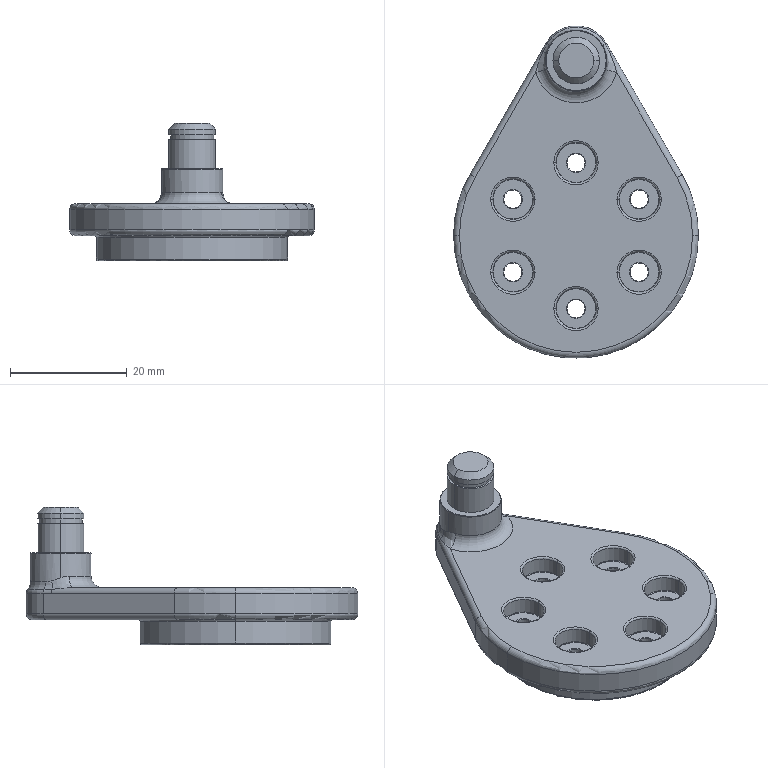Part | SolidWorks | features ICE 7, Fillet 4, Chamfer 1, Extrusion 1 | 1 solid | 129 faces | box 42 x 57 x 23.6 mm | volume 12622 mm3 | torus 64 | cylinder 42 | plane 15 | spline 6 | cone 2 | commonest cylinder face diameters 3.1 x12 7 x12 2 x4 8 x4 42 x3 7.4 x2